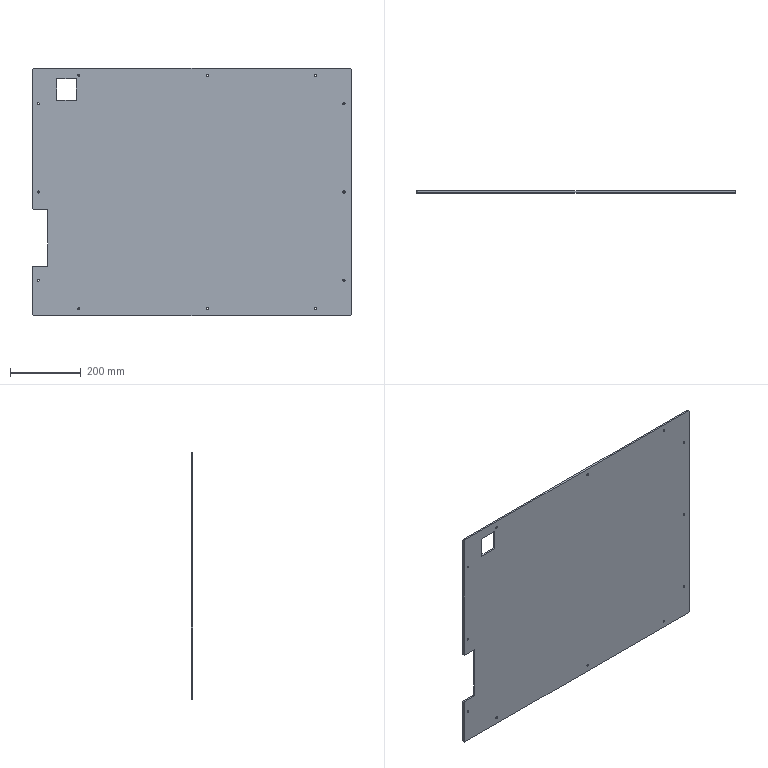Part | STEP file | 227H056117 Top Cover_Default | 1 solid | 44 faces | box 900 x 5 x 700 mm | volume 3097744 mm3 | cylinder 24 | plane 20 | commonest cylinder face diameters 6 x24